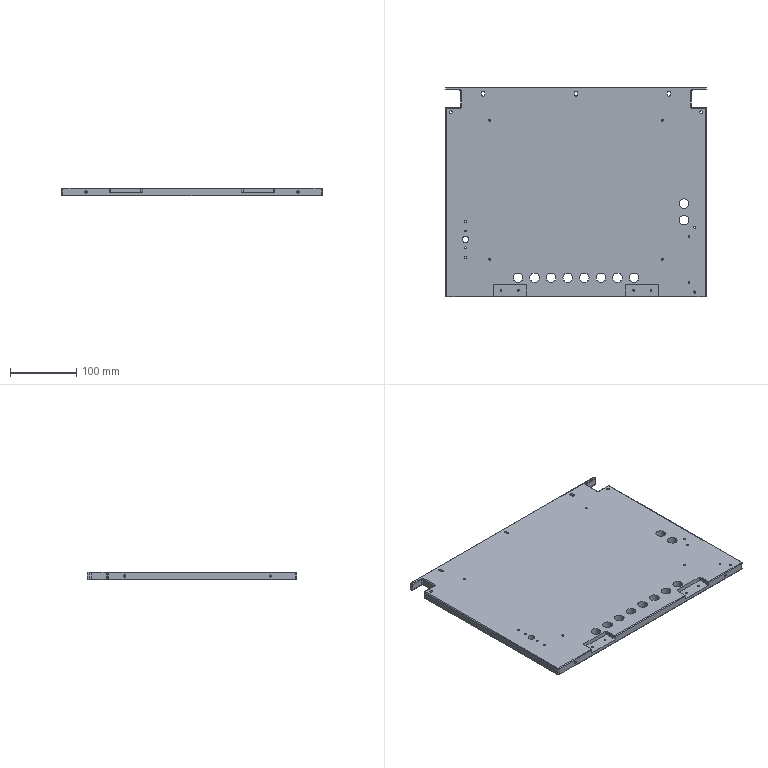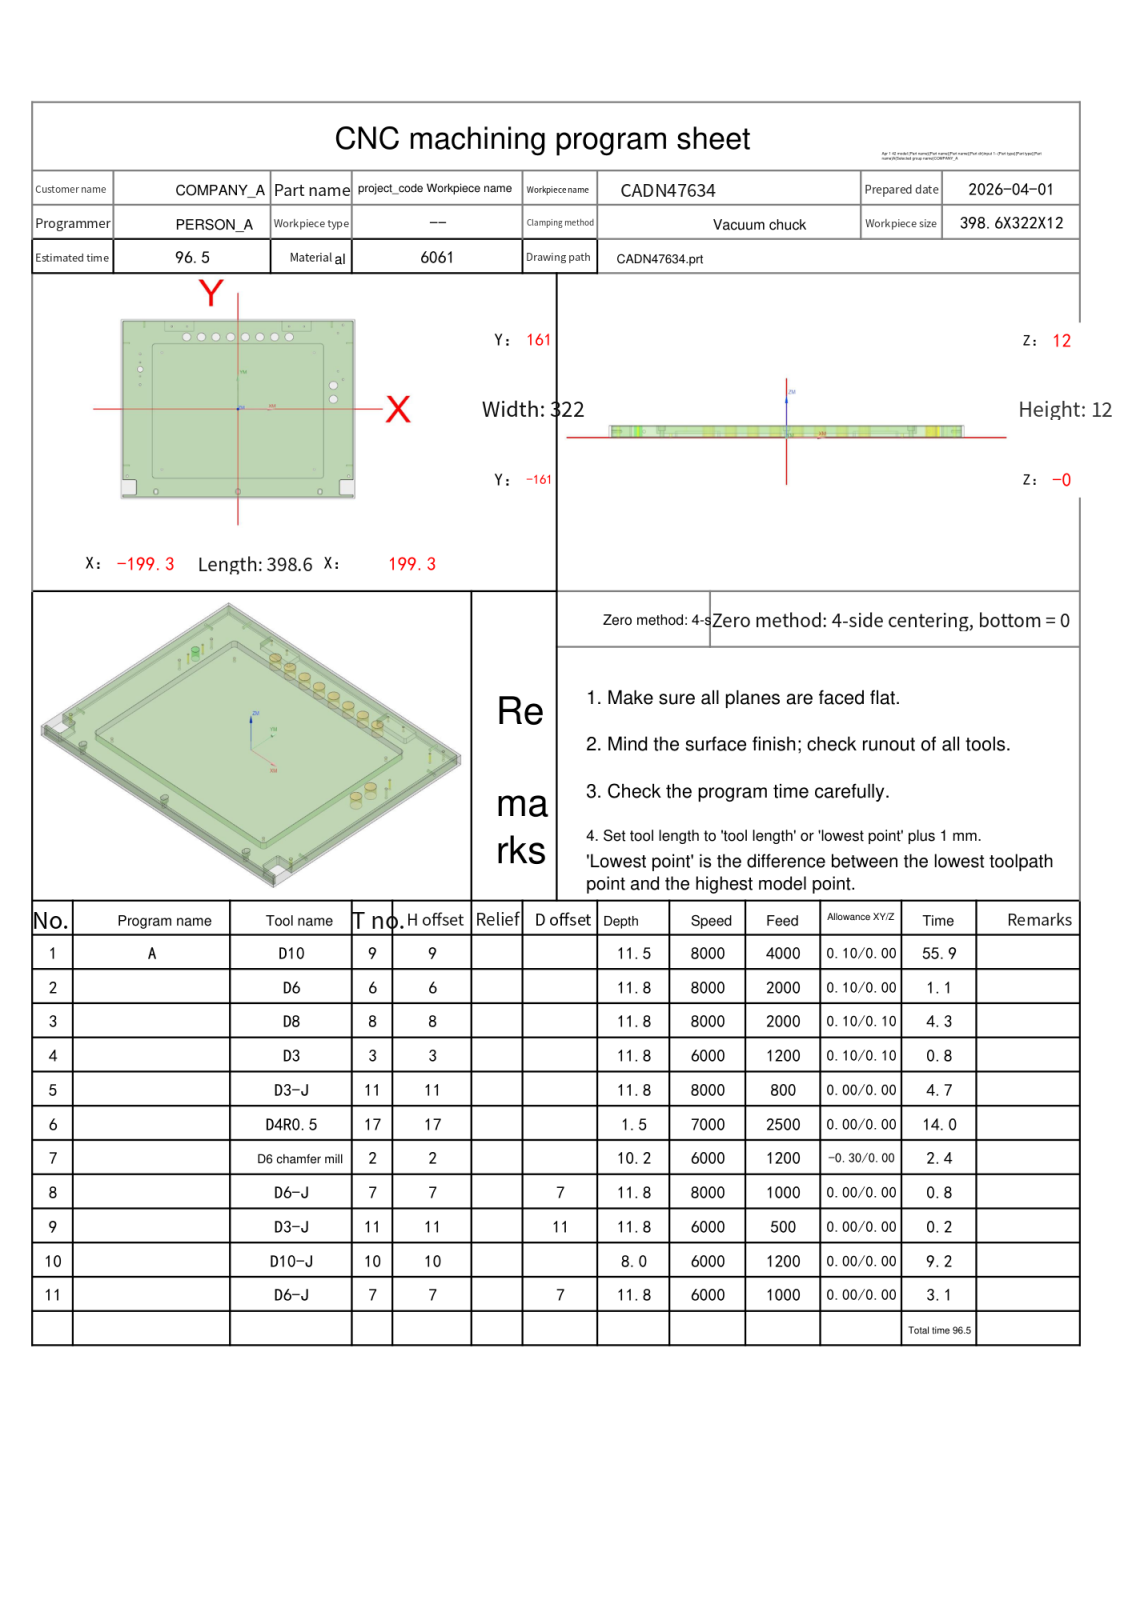NC program | NX | posted by the shop | part box 393.6 x 317 x 12 mm
Lines 5552 to 6526 of 16012:
N5 T11 M06
(D3-J  D=3. R=0. H=11 ce=0.00 di=0.00)
G00 G90 G54 X178.701 Y-128.683 M03 S8000
G43 H11 Z32.
M08
Z12.406
G01 X178.7 Y-128.681 Z12.353 F800.
X178.697 Y-128.675 Z12.3
X178.692 Y-128.665 Z12.245
X178.684 Y-128.652 Z12.191
X178.673 Y-128.637 Z12.138
X178.659 Y-128.621 Z12.087
X178.641 Y-128.604 Z12.038
X178.62 Y-128.588 Z11.994
X178.595 Y-128.572 Z11.953
X178.566 Y-128.557 Z11.919
X178.532 Y-128.544 Z11.89
X178.493 Y-128.534 Z11.869
X178.45 Y-128.528 Z11.855
X178.401 Y-128.526 Z11.851
X175.9
G03 X174.926 Y-129.5 I0.0 J-.974
G01 Y-132.001
X174.939 Y-132.03 Z11.853
X174.978 Y-132.036 Z11.86
X175.039 Y-132.021 Z11.87
X175.121 Y-131.986 Z11.883
X175.221 Y-131.934 Z11.899
X175.337 Y-131.866 Z11.915
X175.606 Y-131.69 Z11.948
X175.783 Y-131.565 Z11.966
X176.075 Y-131.349 Z11.99
X176.525 Y-130.99 Z12.004
X176.976 Y-130.602 Z11.995
X177.413 Y-130.197 Z11.963
X177.82 Y-129.787 Z11.912
X178.067 Y-129.517 Z11.868
X178.209 Y-129.352 Z11.838
X178.413 Y-129.101 Z11.788
X178.492 Y-128.992 Z11.765
X178.554 Y-128.898 Z11.744
X178.597 Y-128.82 Z11.727
X178.618 Y-128.762 Z11.713
X178.616 Y-128.725 Z11.704
X178.588 Y-128.713 Z11.701
X175.9
G03 X175.113 Y-129.5 I0.0 J-.787
G01 Y-132.188
X175.127 Y-132.217 Z11.703
X175.166 Y-132.223 Z11.708
X175.229 Y-132.207 Z11.717
X175.312 Y-132.172 Z11.727
X175.413 Y-132.119 Z11.739
X175.531 Y-132.051 Z11.751
X175.801 Y-131.873 Z11.776
X175.979 Y-131.747 Z11.79
X176.271 Y-131.529 Z11.807
X176.716 Y-131.167 Z11.815
X177.157 Y-130.774 Z11.803
X177.58 Y-130.363 Z11.774
X177.974 Y-129.944 Z11.729
X178.213 Y-129.666 Z11.691
X178.35 Y-129.497 Z11.666
X178.545 Y-129.237 Z11.624
X178.622 Y-129.124 Z11.605
X178.681 Y-129.026 Z11.587
X178.721 Y-128.946 Z11.573
X178.741 Y-128.885 Z11.562
X178.737 Y-128.847 Z11.554
X178.709 Y-128.834 Z11.552
X175.9
G03 X175.234 Y-129.5 I0.0 J-.666
G01 Y-132.309
X175.248 Y-132.338 Z11.553
X175.288 Y-132.345 Z11.557
X175.351 Y-132.33 Z11.563
X175.435 Y-132.297 Z11.571
X175.538 Y-132.246 Z11.579
X175.657 Y-132.179 Z11.588
X175.929 Y-132.005 Z11.606
X176.107 Y-131.881 Z11.615
X176.399 Y-131.665 Z11.625
X176.84 Y-131.301 Z11.627
X177.275 Y-130.905 Z11.613
X177.691 Y-130.487 Z11.586
X178.077 Y-130.058 Z11.547
X178.309 Y-129.773 Z11.515
X178.444 Y-129.599 Z11.494
X178.634 Y-129.332 Z11.461
X178.708 Y-129.215 Z11.445
X178.766 Y-129.114 Z11.431
X178.805 Y-129.031 Z11.419
X178.823 Y-128.968 Z11.41
X178.819 Y-128.929 Z11.405
X178.791 Y-128.915 Z11.403
X175.9
G03 X175.316 Y-129.5 I0.0 J-.585
G01 Y-132.391
X175.33 Y-132.419
X175.37 Y-132.425 Z11.406
X175.434 Y-132.409 Z11.409
X175.518 Y-132.373 Z11.414
X175.622 Y-132.32 Z11.418
X175.741 Y-132.251 Z11.423
X176.014 Y-132.071 Z11.433
X176.192 Y-131.945 Z11.437
X176.484 Y-131.724 Z11.441
X176.923 Y-131.359 Z11.436
X177.353 Y-130.962 Z11.42
X177.764 Y-130.544 Z11.395
X178.143 Y-130.116 Z11.363
X178.372 Y-129.83 Z11.338
X178.504 Y-129.655 Z11.322
X178.691 Y-129.387 Z11.296
X178.764 Y-129.269 Z11.285
X178.82 Y-129.168 Z11.274
X178.858 Y-129.084 Z11.266
X178.876 Y-129.021 Z11.259
X178.871 Y-128.981 Z11.255
X178.843 Y-128.967 Z11.253
X175.9
G03 X175.368 Y-129.5 I0.0 J-.533
G01 Y-132.443
X175.382 Y-132.471
X175.422 Y-132.477 Z11.254
X175.486 Y-132.46 Z11.255
X175.571 Y-132.425 Z11.257
X175.675 Y-132.371 Z11.258
X175.794 Y-132.301 Z11.259
X176.067 Y-132.12 Z11.261
X176.245 Y-131.993 Z11.26
X176.536 Y-131.771 Z11.258
X176.973 Y-131.403 Z11.247
X177.4 Y-131.004 Z11.229
X177.806 Y-130.584 Z11.206
X178.181 Y-130.153 Z11.18
X178.408 Y-129.865 Z11.162
X178.538 Y-129.688 Z11.15
X178.722 Y-129.418 Z11.132
X178.794 Y-129.299 Z11.124
X178.849 Y-129.197 Z11.118
X178.886 Y-129.112 Z11.112
X178.903 Y-129.048 Z11.107
X178.898 Y-129.008 Z11.105
X178.87 Y-128.994 Z11.104
X175.9
G03 X175.395 Y-129.5 I0.0 J-.505
G01 Y-132.47
X175.409 Y-132.498
X175.449 Y-132.503 Z11.103
X175.513 Y-132.487 Z11.102
X175.598 Y-132.451 Z11.101
X175.702 Y-132.396 Z11.099
X175.821 Y-132.326 Z11.097
X176.093 Y-132.144 Z11.091
X176.271 Y-132.016 Z11.087
X176.562 Y-131.793 Z11.078
X176.996 Y-131.422 Z11.062
X177.42 Y-131.021 Z11.044
X177.823 Y-130.598 Z11.024
X178.195 Y-130.165 Z11.003
X178.419 Y-129.875 Z10.991
X178.548 Y-129.697 Z10.983
X178.73 Y-129.426 Z10.972
X178.801 Y-129.307 Z10.967
X178.856 Y-129.203 Z10.962
X178.892 Y-129.118 Z10.959
X178.909 Y-129.054 Z10.957
X178.904 Y-129.014 Z10.955
X178.875 Y-129. Z10.954
X175.9
G03 X175.4 Y-129.5 I0.0 J-.5
G01 Y-132.475
X175.414 Y-132.504
X175.455 Y-132.511 Z10.953
X175.519 Y-132.497 Z10.951
X175.604 Y-132.463 Z10.948
X175.708 Y-132.412 Z10.944
X175.827 Y-132.345 Z10.94
X176.099 Y-132.17 Z10.931
X176.277 Y-132.045 Z10.925
X176.567 Y-131.826 Z10.914
X177.001 Y-131.457 Z10.897
X177.424 Y-131.053 Z10.88
X177.826 Y-130.624 Z10.862
X178.197 Y-130.183 Z10.846
X178.421 Y-129.888 Z10.835
X178.549 Y-129.708 Z10.829
X178.731 Y-129.432 Z10.819
X178.802 Y-129.311 Z10.815
X178.856 Y-129.206 Z10.812
X178.893 Y-129.12 Z10.809
X178.909 Y-129.055 Z10.807
X178.904 Y-129.014 Z10.806
X178.875 Y-129. Z10.805
X175.9
G03 X175.4 Y-129.5 I0.0 J-.5
G01 Y-132.475
X175.414 Y-132.504
X175.455 Y-132.511 Z10.803
X175.519 Y-132.497 Z10.801
X175.604 Y-132.463 Z10.798
X175.708 Y-132.412 Z10.795
X175.827 Y-132.345 Z10.791
X176.099 Y-132.17 Z10.782
X176.277 Y-132.045 Z10.775
X176.567 Y-131.826 Z10.765
X177.001 Y-131.457 Z10.748
X177.424 Y-131.053 Z10.73
X177.826 Y-130.624 Z10.713
X178.197 Y-130.183 Z10.696
X178.421 Y-129.888 Z10.686
X178.549 Y-129.708 Z10.679
X178.731 Y-129.432 Z10.67
X178.802 Y-129.311 Z10.666
X178.856 Y-129.206 Z10.662
X178.893 Y-129.12 Z10.66
X178.909 Y-129.055 Z10.657
X178.904 Y-129.014 Z10.656
X178.875 Y-129.
X175.9
G03 X175.4 Y-129.5 I0.0 J-.5
G01 Y-132.475
X175.414 Y-132.504 Z10.655
X175.455 Y-132.511 Z10.654
X175.519 Y-132.497 Z10.652
X175.604 Y-132.463 Z10.649
X175.708 Y-132.412 Z10.646
X175.827 Y-132.345 Z10.642
X176.099 Y-132.17 Z10.632
X176.277 Y-132.045 Z10.626
X176.567 Y-131.826 Z10.615
X177.001 Y-131.457 Z10.598
X177.424 Y-131.053 Z10.581
X177.826 Y-130.624 Z10.564
X178.197 Y-130.183 Z10.547
X178.421 Y-129.888 Z10.536
X178.549 Y-129.708 Z10.53
X178.731 Y-129.432 Z10.52
X178.802 Y-129.311 Z10.516
X178.856 Y-129.206 Z10.513
X178.893 Y-129.12 Z10.51
X178.909 Y-129.055 Z10.508
X178.904 Y-129.014 Z10.507
X178.875 Y-129. Z10.506
X175.9
G03 X175.4 Y-129.5 I0.0 J-.5
G01 Y-132.475
X175.414 Y-132.504
X175.455 Y-132.511 Z10.505
X175.519 Y-132.497 Z10.502
X175.604 Y-132.463 Z10.5
X175.708 Y-132.412 Z10.496
X175.827 Y-132.345 Z10.492
X176.099 Y-132.17 Z10.483
X176.277 Y-132.045 Z10.476
X176.567 Y-131.826 Z10.466
X177.001 Y-131.457 Z10.449
X177.424 Y-131.053 Z10.432
X177.826 Y-130.624 Z10.414
X178.197 Y-130.183 Z10.397
X178.421 Y-129.888 Z10.387
X178.549 Y-129.708 Z10.381
X178.731 Y-129.432 Z10.371
X178.802 Y-129.311 Z10.367
X178.856 Y-129.206 Z10.364
X178.893 Y-129.12 Z10.361
X178.909 Y-129.055 Z10.359
X178.904 Y-129.014 Z10.357
X178.875 Y-129.
X175.9
G03 X175.4 Y-129.5 I0.0 J-.5
G01 Y-132.475
X175.414 Y-132.504
X175.455 Y-132.511 Z10.355
X175.519 Y-132.497 Z10.353
X175.604 Y-132.463 Z10.35
X175.708 Y-132.412 Z10.347
X175.827 Y-132.345 Z10.343
X176.099 Y-132.17 Z10.333
X176.277 Y-132.045 Z10.327
X176.567 Y-131.826 Z10.317
X177.001 Y-131.457 Z10.3
X177.424 Y-131.053 Z10.282
X177.826 Y-130.624 Z10.265
X178.197 Y-130.183 Z10.248
X178.421 Y-129.888 Z10.237
X178.549 Y-129.708 Z10.231
X178.731 Y-129.432 Z10.222
X178.802 Y-129.311 Z10.218
X178.856 Y-129.206 Z10.214
X178.893 Y-129.12 Z10.211
X178.909 Y-129.055 Z10.209
X178.904 Y-129.014 Z10.208
X178.875 Y-129.
X175.9
G03 X175.4 Y-129.5 I0.0 J-.5
G01 Y-132.475
X175.414 Y-132.504 Z10.207
X175.455 Y-132.511 Z10.206
X175.519 Y-132.497 Z10.204
X175.604 Y-132.463 Z10.201
X175.708 Y-132.412 Z10.197
X175.827 Y-132.345 Z10.193
X176.099 Y-132.17 Z10.184
X176.277 Y-132.045 Z10.178
X176.567 Y-131.826 Z10.167
X177.001 Y-131.457 Z10.15
X177.424 Y-131.053 Z10.133
X177.826 Y-130.624 Z10.116
X178.197 Y-130.183 Z10.099
X178.421 Y-129.888 Z10.088
X178.549 Y-129.708 Z10.082
X178.731 Y-129.432 Z10.072
X178.802 Y-129.311 Z10.068
X178.856 Y-129.206 Z10.065
X178.893 Y-129.12 Z10.062
X178.909 Y-129.055 Z10.06
X178.904 Y-129.014 Z10.059
X178.875 Y-129. Z10.058
X175.9
G03 X175.4 Y-129.5 I0.0 J-.5
G01 Y-132.475
X175.414 Y-132.504
X175.455 Y-132.511 Z10.056
X175.519 Y-132.497 Z10.054
X175.604 Y-132.463 Z10.052
X175.708 Y-132.412 Z10.048
X175.827 Y-132.345 Z10.044
X176.099 Y-132.17 Z10.035
X176.277 Y-132.045 Z10.028
X176.567 Y-131.826 Z10.018
X177.001 Y-131.457 Z10.001
X177.424 Y-131.053 Z9.984
X177.826 Y-130.624 Z9.966
X178.197 Y-130.183 Z9.949
X178.421 Y-129.888 Z9.939
X178.549 Y-129.708 Z9.932
X178.731 Y-129.432 Z9.923
X178.802 Y-129.311 Z9.919
X178.856 Y-129.206 Z9.916
X178.893 Y-129.12 Z9.913
X178.909 Y-129.055 Z9.911
X178.904 Y-129.014 Z9.909
X178.875 Y-129.
X175.9
G03 X175.4 Y-129.5 I0.0 J-.5
G01 Y-132.475
X175.414 Y-132.504 Z9.908
X175.455 Y-132.511 Z9.907
X175.519 Y-132.497 Z9.905
X175.604 Y-132.463 Z9.902
X175.708 Y-132.412 Z9.899
X175.827 Y-132.345 Z9.895
X176.099 Y-132.17 Z9.885
X176.277 Y-132.045 Z9.879
X176.567 Y-131.826 Z9.868
X177.001 Y-131.457 Z9.852
X177.424 Y-131.053 Z9.834
X177.826 Y-130.624 Z9.817
X178.197 Y-130.183 Z9.8
X178.421 Y-129.888 Z9.789
X178.549 Y-129.708 Z9.783
X178.731 Y-129.432 Z9.774
X178.802 Y-129.311 Z9.77
X178.856 Y-129.206 Z9.766
X178.893 Y-129.12 Z9.763
X178.909 Y-129.055 Z9.761
X178.904 Y-129.014 Z9.76
X178.875 Y-129. Z9.759
X175.9
G03 X175.4 Y-129.5 I0.0 J-.5
G01 Y-132.475
X175.414 Y-132.504
X175.455 Y-132.511 Z9.758
X175.519 Y-132.497 Z9.756
X175.604 Y-132.463 Z9.753
X175.708 Y-132.412 Z9.749
X175.827 Y-132.345 Z9.745
X176.099 Y-132.17 Z9.736
X176.277 Y-132.045 Z9.73
X176.567 Y-131.826 Z9.719
X177.001 Y-131.457 Z9.702
X177.424 Y-131.053 Z9.685
X177.826 Y-130.624 Z9.667
X178.197 Y-130.183 Z9.651
X178.421 Y-129.888 Z9.64
X178.549 Y-129.708 Z9.634
X178.731 Y-129.432 Z9.624
X178.802 Y-129.311 Z9.62
X178.856 Y-129.206 Z9.617
X178.893 Y-129.12 Z9.614
X178.909 Y-129.055 Z9.612
X178.904 Y-129.014 Z9.611
X178.875 Y-129. Z9.61
X175.9
G03 X175.4 Y-129.5 I0.0 J-.5
G01 Y-132.475
X175.414 Y-132.504
X175.455 Y-132.511 Z9.608
X175.519 Y-132.497 Z9.606
X175.604 Y-132.463 Z9.603
X175.708 Y-132.412 Z9.6
X175.827 Y-132.345 Z9.596
X176.099 Y-132.17 Z9.587
X176.277 Y-132.045 Z9.58
X176.567 Y-131.826 Z9.57
X177.001 Y-131.457 Z9.553
X177.424 Y-131.053 Z9.535
X177.826 Y-130.624 Z9.518
X178.197 Y-130.183 Z9.501
X178.421 Y-129.888 Z9.491
X178.549 Y-129.708 Z9.484
X178.731 Y-129.432 Z9.475
X178.802 Y-129.311 Z9.471
X178.856 Y-129.206 Z9.467
X178.893 Y-129.12 Z9.465
X178.909 Y-129.055 Z9.463
X178.904 Y-129.014 Z9.461
X178.875 Y-129.
X175.9
G03 X175.4 Y-129.5 I0.0 J-.5
G01 Y-132.475
X175.414 Y-132.504 Z9.46
X175.455 Y-132.511 Z9.459
X175.519 Y-132.497 Z9.457
X175.604 Y-132.463 Z9.454
X175.708 Y-132.412 Z9.451
X175.827 Y-132.345 Z9.447
X176.099 Y-132.17 Z9.437
X176.277 Y-132.045 Z9.431
X176.567 Y-131.826 Z9.42
X177.001 Y-131.457 Z9.403
X177.424 Y-131.053 Z9.386
X177.826 Y-130.624 Z9.369
X178.197 Y-130.183 Z9.352
X178.421 Y-129.888 Z9.341
X178.549 Y-129.708 Z9.335
X178.731 Y-129.432 Z9.326
X178.802 Y-129.311 Z9.322
X178.856 Y-129.206 Z9.318
X178.893 Y-129.12 Z9.315
X178.909 Y-129.055 Z9.313
X178.904 Y-129.014 Z9.312
X178.875 Y-129. Z9.311
X175.9
G03 X175.4 Y-129.5 I0.0 J-.5
G01 Y-132.475
X175.414 Y-132.504
X175.455 Y-132.511 Z9.31
X175.519 Y-132.497 Z9.308
X175.604 Y-132.463 Z9.305
X175.708 Y-132.412 Z9.301
X175.827 Y-132.345 Z9.297
X176.099 Y-132.17 Z9.288
X176.277 Y-132.045 Z9.282
X176.567 Y-131.826 Z9.271
X177.001 Y-131.457 Z9.254
X177.424 Y-131.053 Z9.237
X177.826 Y-130.624 Z9.219
X178.197 Y-130.183 Z9.202
X178.421 Y-129.888 Z9.192
X178.549 Y-129.708 Z9.186
X178.731 Y-129.432 Z9.176
X178.802 Y-129.311 Z9.172
X178.856 Y-129.206 Z9.169
X178.893 Y-129.12 Z9.166
X178.909 Y-129.055 Z9.164
X178.904 Y-129.014 Z9.162
X178.875 Y-129.
X175.9
G03 X175.4 Y-129.5 I0.0 J-.5
G01 Y-132.475
X175.414 Y-132.504
X175.455 Y-132.511 Z9.16
X175.519 Y-132.497 Z9.158
X175.604 Y-132.463 Z9.155
X175.708 Y-132.412 Z9.152
X175.827 Y-132.345 Z9.148
X176.099 Y-132.17 Z9.138
X176.277 Y-132.045 Z9.132
X176.567 Y-131.826 Z9.122
X177.001 Y-131.457 Z9.105
X177.424 Y-131.053 Z9.087
X177.826 Y-130.624 Z9.07
X178.197 Y-130.183 Z9.053
X178.421 Y-129.888 Z9.043
X178.549 Y-129.708 Z9.036
X178.731 Y-129.432 Z9.027
X178.802 Y-129.311 Z9.023
X178.856 Y-129.206 Z9.019
X178.893 Y-129.12 Z9.017
X178.909 Y-129.055 Z9.014
X178.904 Y-129.014 Z9.013
X178.875 Y-129.
X175.9
G03 X175.4 Y-129.5 I0.0 J-.5
G01 Y-132.475
X175.414 Y-132.504 Z9.012
X175.455 Y-132.511 Z9.011
X175.519 Y-132.497 Z9.009
X175.604 Y-132.463 Z9.006
X175.708 Y-132.412 Z9.003
X175.827 Y-132.345 Z8.999
X176.099 Y-132.17 Z8.989
X176.277 Y-132.045 Z8.983
X176.567 Y-131.826 Z8.972
X177.001 Y-131.457 Z8.955
X177.424 Y-131.053 Z8.938
X177.826 Y-130.624 Z8.921
X178.197 Y-130.183 Z8.904
X178.421 Y-129.888 Z8.893
X178.549 Y-129.708 Z8.887
X178.731 Y-129.432 Z8.877
X178.802 Y-129.311 Z8.873
X178.856 Y-129.206 Z8.87
X178.893 Y-129.12 Z8.867
X178.909 Y-129.055 Z8.865
X178.904 Y-129.014 Z8.864
X178.875 Y-129. Z8.863
X175.9
G03 X175.4 Y-129.5 I0.0 J-.5
G01 Y-132.475
X175.414 Y-132.504
X175.455 Y-132.511 Z8.862
X175.519 Y-132.497 Z8.859
X175.604 Y-132.463 Z8.857
X175.708 Y-132.412 Z8.853
X175.827 Y-132.345 Z8.849
X176.099 Y-132.17 Z8.84
X176.277 Y-132.045 Z8.833
X176.567 Y-131.826 Z8.823
X177.001 Y-131.457 Z8.806
X177.424 Y-131.053 Z8.789
X177.826 Y-130.624 Z8.771
X178.197 Y-130.183 Z8.754
X178.421 Y-129.888 Z8.744
X178.549 Y-129.708 Z8.737
X178.731 Y-129.432 Z8.728
X178.802 Y-129.311 Z8.724
X178.856 Y-129.206 Z8.721
X178.893 Y-129.12 Z8.718
X178.909 Y-129.055 Z8.716
X178.904 Y-129.014 Z8.714
X178.875 Y-129.
X175.9
G03 X175.4 Y-129.5 I0.0 J-.5
G01 Y-132.475
X175.414 Y-132.504 Z8.713
X175.455 Y-132.511 Z8.712
X175.519 Y-132.497 Z8.71
X175.604 Y-132.463 Z8.707
X175.708 Y-132.412 Z8.704
X175.827 Y-132.345 Z8.7
X176.099 Y-132.17 Z8.69
X176.277 Y-132.045 Z8.684
X176.567 Y-131.826 Z8.673
X177.001 Y-131.457 Z8.657
X177.424 Y-131.053 Z8.639
X177.826 Y-130.624 Z8.622
X178.197 Y-130.183 Z8.605
X178.421 Y-129.888 Z8.594
X178.549 Y-129.708 Z8.588
X178.731 Y-129.432 Z8.579
X178.802 Y-129.311 Z8.575
X178.856 Y-129.206 Z8.571
X178.893 Y-129.12 Z8.568
X178.909 Y-129.055 Z8.566
X178.904 Y-129.014 Z8.565
X178.875 Y-129.
X175.9
G03 X175.4 Y-129.5 I0.0 J-.5
G01 Y-132.475
X175.414 Y-132.504 Z8.564
X175.455 Y-132.511 Z8.563
X175.519 Y-132.497 Z8.561
X175.604 Y-132.463 Z8.558
X175.708 Y-132.412 Z8.554
X175.827 Y-132.345 Z8.55
X176.099 Y-132.17 Z8.541
X176.277 Y-132.045 Z8.535
X176.567 Y-131.826 Z8.524
X177.001 Y-131.457 Z8.507
X177.424 Y-131.053 Z8.49
X177.826 Y-130.624 Z8.472
X178.197 Y-130.183 Z8.456
X178.421 Y-129.888 Z8.445
X178.549 Y-129.708 Z8.439
X178.731 Y-129.432 Z8.429
X178.802 Y-129.311 Z8.425
X178.856 Y-129.206 Z8.422
X178.893 Y-129.12 Z8.419
X178.909 Y-129.055 Z8.417
X178.904 Y-129.014 Z8.416
X178.875 Y-129. Z8.415
X175.9
G03 X175.4 Y-129.5 I0.0 J-.5
G01 Y-132.475
X175.414 Y-132.504
X175.455 Y-132.511 Z8.413
X175.519 Y-132.497 Z8.411
X175.604 Y-132.463 Z8.409
X175.708 Y-132.412 Z8.405
X175.827 Y-132.345 Z8.401
X176.099 Y-132.17 Z8.392
X176.277 Y-132.045 Z8.385
X176.567 Y-131.826 Z8.375
X177.001 Y-131.457 Z8.358
X177.424 Y-131.053 Z8.341
X177.826 Y-130.624 Z8.323
X178.197 Y-130.183 Z8.306
X178.421 Y-129.888 Z8.296
X178.549 Y-129.708 Z8.289
X178.731 Y-129.432 Z8.28
X178.802 Y-129.311 Z8.276
X178.856 Y-129.206 Z8.272
X178.893 Y-129.12 Z8.27
X178.909 Y-129.055 Z8.268
X178.904 Y-129.014 Z8.266
X178.875 Y-129.
X175.9
G03 X175.4 Y-129.5 I0.0 J-.5
G01 Y-132.475
X175.414 Y-132.504 Z8.265
X175.455 Y-132.511 Z8.264
X175.519 Y-132.497 Z8.262
X175.604 Y-132.463 Z8.259
X175.708 Y-132.412 Z8.256
X175.827 Y-132.345 Z8.252
X176.099 Y-132.17 Z8.242
X176.277 Y-132.045 Z8.236
X176.567 Y-131.826 Z8.225
X177.001 Y-131.457 Z8.209
X177.424 Y-131.053 Z8.191
X177.826 Y-130.624 Z8.174
X178.197 Y-130.183 Z8.157
X178.421 Y-129.888 Z8.146
X178.549 Y-129.708 Z8.14
X178.731 Y-129.432 Z8.131
X178.802 Y-129.311 Z8.127
X178.856 Y-129.206 Z8.123
X178.893 Y-129.12 Z8.12
X178.909 Y-129.055 Z8.118
X178.904 Y-129.014 Z8.117
X178.875 Y-129. Z8.116
X175.9
G03 X175.4 Y-129.5 I0.0 J-.5
G01 Y-132.475
X175.414 Y-132.504
X175.455 Y-132.511 Z8.115
X175.519 Y-132.497 Z8.113
X175.604 Y-132.463 Z8.11
X175.708 Y-132.412 Z8.106
X175.827 Y-132.345 Z8.102
X176.099 Y-132.17 Z8.093
X176.277 Y-132.045 Z8.087
X176.567 Y-131.826 Z8.076
X177.001 Y-131.457 Z8.059
X177.424 Y-131.053 Z8.042
X177.826 Y-130.624 Z8.024
X178.197 Y-130.183 Z8.008
X178.421 Y-129.888 Z7.997
X178.549 Y-129.708 Z7.991
X178.731 Y-129.432 Z7.981
X178.802 Y-129.311 Z7.977
X178.856 Y-129.206 Z7.974
X178.893 Y-129.12 Z7.971
X178.909 Y-129.055 Z7.969
X178.904 Y-129.014 Z7.968
X178.875 Y-129. Z7.967
X175.9
G03 X175.4 Y-129.5 I0.0 J-.5
G01 Y-132.475
X175.414 Y-132.504
X175.455 Y-132.511 Z7.965
X175.519 Y-132.497 Z7.963
X175.604 Y-132.463 Z7.96
X175.708 Y-132.412 Z7.957
X175.827 Y-132.345 Z7.953
X176.099 Y-132.17 Z7.944
X176.277 Y-132.045 Z7.937
X176.567 Y-131.826 Z7.927
X177.001 Y-131.457 Z7.91
X177.424 Y-131.053 Z7.892
X177.826 Y-130.624 Z7.875
X178.197 Y-130.183 Z7.858
X178.421 Y-129.888 Z7.848
X178.549 Y-129.708 Z7.841
X178.731 Y-129.432 Z7.832
X178.802 Y-129.311 Z7.828
X178.856 Y-129.206 Z7.824
X178.893 Y-129.12 Z7.822
X178.909 Y-129.055 Z7.819
X178.904 Y-129.014 Z7.818
X178.875 Y-129.
X175.9
G03 X175.4 Y-129.5 I0.0 J-.5
G01 Y-132.475
X175.414 Y-132.504 Z7.817
X175.455 Y-132.511 Z7.816
X175.519 Y-132.497 Z7.814
X175.604 Y-132.463 Z7.811
X175.708 Y-132.412 Z7.808
X175.827 Y-132.345 Z7.804
X176.099 Y-132.17 Z7.794
X176.277 Y-132.045 Z7.788
X176.567 Y-131.826 Z7.777
X177.001 Y-131.457 Z7.76
X177.424 Y-131.053 Z7.743
X177.826 Y-130.624 Z7.726
X178.197 Y-130.183 Z7.709
X178.421 Y-129.888 Z7.698
X178.549 Y-129.708 Z7.692
X178.731 Y-129.432 Z7.682
X178.802 Y-129.311 Z7.678
X178.856 Y-129.206 Z7.675
X178.893 Y-129.12 Z7.672
X178.909 Y-129.055 Z7.67
X178.904 Y-129.014 Z7.669
X178.875 Y-129. Z7.668
X175.9
G03 X175.4 Y-129.5 I0.0 J-.5
G01 Y-132.475
X175.414 Y-132.504
X175.455 Y-132.511 Z7.667
X175.519 Y-132.497 Z7.665
X175.604 Y-132.463 Z7.662
X175.708 Y-132.412 Z7.658
X175.827 Y-132.345 Z7.654
X176.099 Y-132.17 Z7.645
X176.277 Y-132.045 Z7.638
X176.567 Y-131.826 Z7.628
X177.001 Y-131.457 Z7.611
X177.424 Y-131.053 Z7.594
X177.826 Y-130.624 Z7.576
X178.197 Y-130.183 Z7.559
X178.421 Y-129.888 Z7.549
X178.549 Y-129.708 Z7.543
X178.731 Y-129.432 Z7.533
X178.802 Y-129.311 Z7.529
X178.856 Y-129.206 Z7.526
X178.893 Y-129.12 Z7.523
X178.909 Y-129.055 Z7.521
X178.904 Y-129.014 Z7.519
X178.875 Y-129.
X175.9
G03 X175.4 Y-129.5 I0.0 J-.5
G01 Y-132.475
X175.414 Y-132.504
X175.455 Y-132.511 Z7.517
X175.519 Y-132.497 Z7.515
X175.604 Y-132.463 Z7.512
X175.708 Y-132.412 Z7.509
X175.827 Y-132.345 Z7.505
X176.099 Y-132.17 Z7.495
X176.277 Y-132.045 Z7.489
X176.567 Y-131.826 Z7.479
X177.001 Y-131.457 Z7.462
X177.424 Y-131.053 Z7.444
X177.826 Y-130.624 Z7.427
X178.197 Y-130.183 Z7.41
X178.421 Y-129.888 Z7.399
X178.549 Y-129.708 Z7.393
X178.731 Y-129.432 Z7.384
X178.802 Y-129.311 Z7.38
X178.856 Y-129.206 Z7.376
X178.893 Y-129.12 Z7.373
X178.909 Y-129.055 Z7.371
X178.904 Y-129.014 Z7.37
X178.875 Y-129.
X175.9
G03 X175.4 Y-129.5 I0.0 J-.5
G01 Y-132.475
X175.414 Y-132.504 Z7.369
X175.455 Y-132.511 Z7.368
X175.519 Y-132.497 Z7.366
X175.604 Y-132.463 Z7.363
X175.708 Y-132.412 Z7.36
X175.827 Y-132.345 Z7.355
X176.099 Y-132.17 Z7.346
X176.277 Y-132.045 Z7.34
X176.567 Y-131.826 Z7.329
X177.001 Y-131.457 Z7.312
X177.424 Y-131.053 Z7.295
X177.826 Y-130.624 Z7.278
X178.197 Y-130.183 Z7.261
X178.421 Y-129.888 Z7.25
X178.549 Y-129.708 Z7.244
X178.731 Y-129.432 Z7.234
X178.802 Y-129.311 Z7.23
X178.856 Y-129.206 Z7.227
X178.893 Y-129.12 Z7.224
X178.909 Y-129.055 Z7.222
X178.904 Y-129.014 Z7.221
X178.875 Y-129. Z7.22
X175.9
G03 X175.4 Y-129.5 I0.0 J-.5
G01 Y-132.475
X175.414 Y-132.504
X175.455 Y-132.511 Z7.218
X175.519 Y-132.497 Z7.216
X175.604 Y-132.463 Z7.214
X175.708 Y-132.412 Z7.21
X175.827 Y-132.345 Z7.206
X176.099 Y-132.17 Z7.197
X176.277 Y-132.045 Z7.19
X176.567 Y-131.826 Z7.18
X177.001 Y-131.457 Z7.163
X177.424 Y-131.053 Z7.146
X177.826 Y-130.624 Z7.128
X178.197 Y-130.183 Z7.111
X178.421 Y-129.888 Z7.101
X178.549 Y-129.708 Z7.094
X178.731 Y-129.432 Z7.085
X178.802 Y-129.311 Z7.081
X178.856 Y-129.206 Z7.078
X178.893 Y-129.12 Z7.075
X178.909 Y-129.055 Z7.073
X178.904 Y-129.014 Z7.071
X178.875 Y-129.
X175.9
G03 X175.4 Y-129.5 I0.0 J-.5
G01 Y-132.475
X175.414 Y-132.504 Z7.07
X175.455 Y-132.511 Z7.069
X175.519 Y-132.497 Z7.067
X175.604 Y-132.463 Z7.064
X175.708 Y-132.412 Z7.061
X175.827 Y-132.345 Z7.057
X176.099 Y-132.17 Z7.047
X176.277 Y-132.045 Z7.041
X176.567 Y-131.826 Z7.03
X177.001 Y-131.457 Z7.014
X177.424 Y-131.053 Z6.996
X177.826 Y-130.624 Z6.979
X178.197 Y-130.183 Z6.962
X178.421 Y-129.888 Z6.951
X178.549 Y-129.708 Z6.945
X178.731 Y-129.432 Z6.936
X178.802 Y-129.311 Z6.932
X178.856 Y-129.206 Z6.928
X178.893 Y-129.12 Z6.925
X178.909 Y-129.055 Z6.923
X178.904 Y-129.014 Z6.922
X178.875 Y-129.
X175.9
G03 X175.4 Y-129.5 I0.0 J-.5
G01 Y-132.475
X175.414 Y-132.504 Z6.921
X175.455 Y-132.511 Z6.92
X175.519 Y-132.497 Z6.918
X175.604 Y-132.463 Z6.915
X175.708 Y-132.412 Z6.911
X175.827 Y-132.345 Z6.907
X176.099 Y-132.17 Z6.898
X176.277 Y-132.045 Z6.892
X176.567 Y-131.826 Z6.881
X177.001 Y-131.457 Z6.864
X177.424 Y-131.053 Z6.847
X177.826 Y-130.624 Z6.829
X178.197 Y-130.183 Z6.813
X178.421 Y-129.888 Z6.802
X178.549 Y-129.708 Z6.796
X178.731 Y-129.432 Z6.786
X178.802 Y-129.311 Z6.782
X178.856 Y-129.206 Z6.779
X178.893 Y-129.12 Z6.776
X178.909 Y-129.055 Z6.774
X178.904 Y-129.014 Z6.773
X178.875 Y-129. Z6.772
X175.9
G03 X175.4 Y-129.5 I0.0 J-.5
G01 Y-132.475
X175.414 Y-132.504
X175.455 Y-132.511 Z6.77
X175.519 Y-132.497 Z6.768
X175.604 Y-132.463 Z6.765
X175.708 Y-132.412 Z6.762
X175.827 Y-132.345 Z6.758
X176.099 Y-132.17 Z6.749
X176.277 Y-132.045 Z6.742
X176.567 Y-131.826 Z6.732
X177.001 Y-131.457 Z6.715
X177.424 Y-131.053 Z6.697
X177.826 Y-130.624 Z6.68
X178.197 Y-130.183 Z6.663
X178.421 Y-129.888 Z6.653
X178.549 Y-129.708 Z6.646
X178.731 Y-129.432 Z6.637
X178.802 Y-129.311 Z6.633
X178.856 Y-129.206 Z6.629
X178.893 Y-129.12 Z6.627
X178.909 Y-129.055 Z6.625
X178.904 Y-129.014 Z6.623
X178.875 Y-129.
X175.9
G03 X175.4 Y-129.5 I0.0 J-.5
G01 Y-132.475
X175.414 Y-132.504 Z6.622
X175.455 Y-132.511 Z6.621
X175.519 Y-132.497 Z6.619
X175.604 Y-132.463 Z6.616
X175.708 Y-132.412 Z6.613
X175.827 Y-132.345 Z6.609
X176.099 Y-132.17 Z6.599
X176.277 Y-132.045 Z6.593
X176.567 Y-131.826 Z6.582
X177.001 Y-131.457 Z6.566
X177.424 Y-131.053 Z6.548
X177.826 Y-130.624 Z6.531
X178.197 Y-130.183 Z6.514
X178.421 Y-129.888 Z6.503
X178.549 Y-129.708 Z6.497
X178.731 Y-129.432 Z6.488
X178.802 Y-129.311 Z6.484
X178.856 Y-129.206 Z6.48
X178.893 Y-129.12 Z6.477
X178.909 Y-129.055 Z6.475
X178.904 Y-129.014 Z6.474
X178.875 Y-129. Z6.473
X175.9
G03 X175.4 Y-129.5 I0.0 J-.5
G01 Y-132.475
X175.414 Y-132.504
X175.455 Y-132.511 Z6.472
X175.519 Y-132.497 Z6.47
X175.604 Y-132.463 Z6.467
X175.708 Y-132.412 Z6.463
X175.827 Y-132.345 Z6.459
X176.099 Y-132.17 Z6.45
X176.277 Y-132.045 Z6.444
X176.567 Y-131.826 Z6.433
X177.001 Y-131.457 Z6.416
X177.424 Y-131.053 Z6.399
X177.826 Y-130.624 Z6.381
X178.197 Y-130.183 Z6.365
X178.421 Y-129.888 Z6.354
X178.549 Y-129.708 Z6.348
X178.731 Y-129.432 Z6.338
X178.802 Y-129.311 Z6.334
X178.856 Y-129.206 Z6.331
X178.893 Y-129.12 Z6.328
X178.909 Y-129.055 Z6.326
X178.904 Y-129.014 Z6.325
X178.875 Y-129. Z6.324
X175.9
G03 X175.4 Y-129.5 I0.0 J-.5
G01 Y-132.475
X175.414 Y-132.504
X175.455 Y-132.511 Z6.322
X175.519 Y-132.497 Z6.32
X175.604 Y-132.463 Z6.317
X175.708 Y-132.412 Z6.314
X175.827 Y-132.345 Z6.31
X176.099 Y-132.17 Z6.3
X176.277 Y-132.045 Z6.294
X176.567 Y-131.826 Z6.284
X177.001 Y-131.457 Z6.267
X177.424 Y-131.053 Z6.249
X177.826 Y-130.624 Z6.232
X178.197 Y-130.183 Z6.215
X178.421 Y-129.888 Z6.205
X178.549 Y-129.708 Z6.198
X178.731 Y-129.432 Z6.189
X178.802 Y-129.311 Z6.185
X178.856 Y-129.206 Z6.181
X178.893 Y-129.12 Z6.179
X178.909 Y-129.055 Z6.176
X178.904 Y-129.014 Z6.175
X178.875 Y-129.
X175.9
G03 X175.4 Y-129.5 I0.0 J-.5
G01 Y-132.475
X175.414 Y-132.504 Z6.174
X175.455 Y-132.511 Z6.173